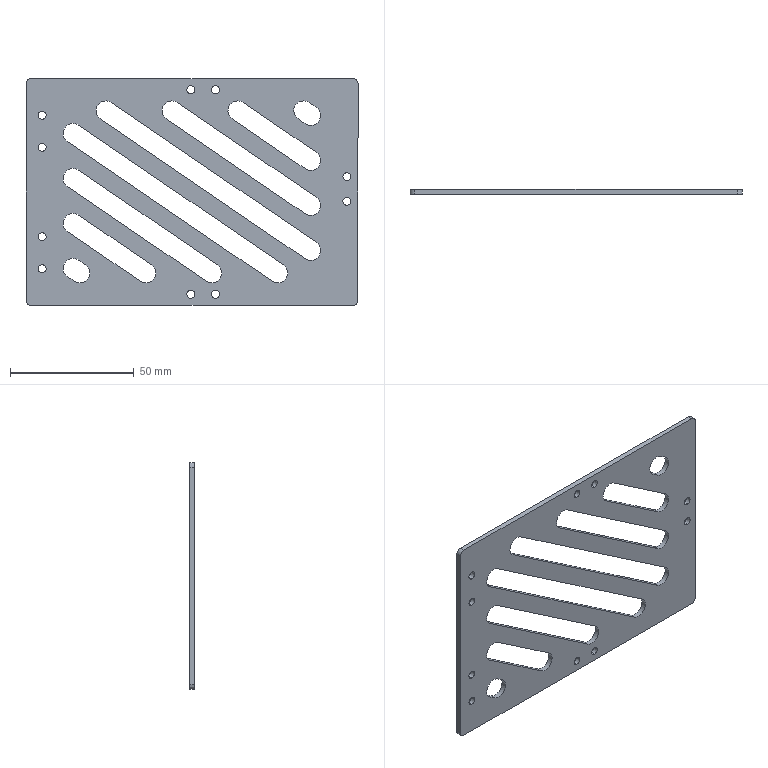Part | SolidWorks | features Fillet 4, ICE 2, Extrusion 1 | 1 solid | 70 faces | box 134 x 2 x 91.5 mm | volume 16934 mm3 | cylinder 48 | plane 22 | commonest cylinder face diameters 8 x24 3.2 x20 4 x4